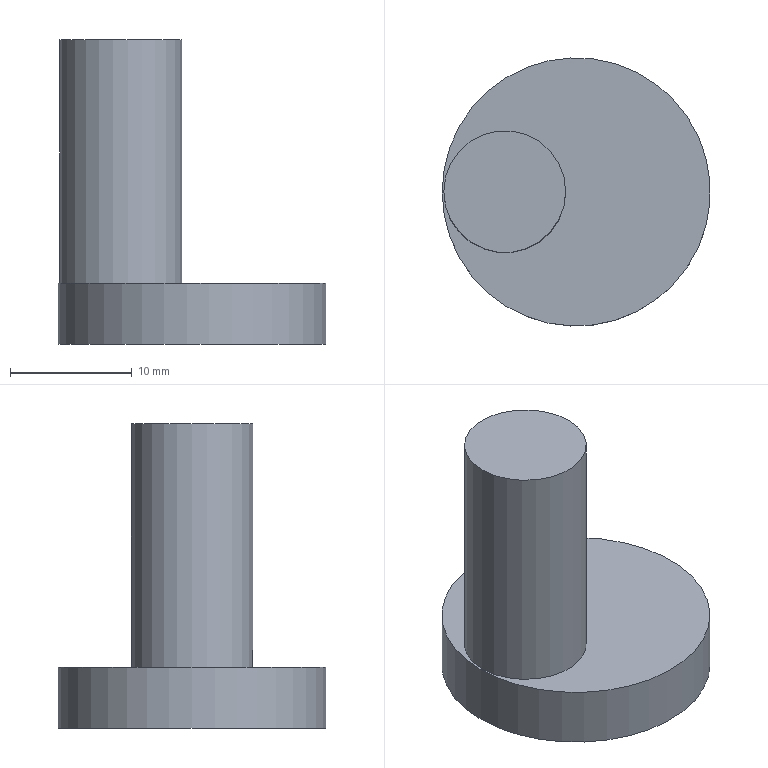Part | STEP file | CMT7E v7 | 1 solid | 5 faces | box 22 x 22 x 25 mm | volume 3472 mm3 | plane 3 | cylinder 2 | commonest cylinder face diameters 10 x1 22 x1
STEP:
#1=CARTESIAN_POINT('',(0.,0.,0.));
#2=DIRECTION('',(0.,0.,1.));
#3=DIRECTION('',(1.,0.,0.));
#4=AXIS2_PLACEMENT_3D('',#1,#2,#3);
#5=CARTESIAN_POINT('',(-79.635,-9.,16.));
#6=VERTEX_POINT('',#5);
#7=CARTESIAN_POINT('',(-68.635,-9.,16.));
#8=DIRECTION('',(0.,0.,1.));
#9=DIRECTION('',(-1.,0.,0.));
#10=AXIS2_PLACEMENT_3D('',#7,#8,#9);
#11=CIRCLE('',#10,11.);
#12=CARTESIAN_POINT('',(-68.635,-9.,16.));
#13=DIRECTION('',(0.,0.,1.));
#14=DIRECTION('',(-1.,0.,0.));
#15=AXIS2_PLACEMENT_3D('',#12,#13,#14);
#16=PLANE('',#15);
#17=CARTESIAN_POINT('',(0.,0.));
#18=DIRECTION('',(1.,0.));
#19=AXIS2_PLACEMENT_2D('',#17,#18);
#20=CIRCLE('',#19,11.);
#21=(GEOMETRIC_REPRESENTATION_CONTEXT(2)PARAMETRIC_REPRESENTATION_CONTEXT()REPRESENTATION_CONTEXT('',''));
#22=DEFINITIONAL_REPRESENTATION('',(#20),#21);
#23=PCURVE('',#16,#22);
#24=CARTESIAN_POINT('',(-68.635,-9.,16.));
#25=DIRECTION('',(0.,0.,1.));
#26=DIRECTION('',(-1.,0.,0.));
#27=AXIS2_PLACEMENT_3D('',#24,#25,#26);
#28=CYLINDRICAL_SURFACE('',#27,11.);
#29=CARTESIAN_POINT('',(0.,0.));
#30=DIRECTION('',(1.,0.));
#31=VECTOR('',#30,1.);
#32=LINE('',#29,#31);
#33=(GEOMETRIC_REPRESENTATION_CONTEXT(2)PARAMETRIC_REPRESENTATION_CONTEXT()REPRESENTATION_CONTEXT('',''));
#34=DEFINITIONAL_REPRESENTATION('',(#32),#33);
#35=PCURVE('',#28,#34);
#36=SURFACE_CURVE('',#11,(#23,#35),.PCURVE_S1.);
#37=EDGE_CURVE('',#6,#6,#36,.T.);
#38=ORIENTED_EDGE('',*,*,#37,.F.);
#39=EDGE_LOOP('',(#38));
#40=FACE_BOUND('',#39,.T.);
#41=ADVANCED_FACE('',(#40),#16,.F.);
#42=CARTESIAN_POINT('',(-79.5,-9.,21.));
#43=VERTEX_POINT('',#42);
#44=CARTESIAN_POINT('',(-74.5,-9.,21.));
#45=DIRECTION('',(0.,0.,-1.));
#46=DIRECTION('',(-1.,0.,0.));
#47=AXIS2_PLACEMENT_3D('',#44,#45,#46);
#48=CIRCLE('',#47,5.);
#49=CARTESIAN_POINT('',(-68.635,-9.,21.));
#50=DIRECTION('',(0.,0.,1.));
#51=DIRECTION('',(-1.,0.,0.));
#52=AXIS2_PLACEMENT_3D('',#49,#50,#51);
#53=PLANE('',#52);
#54=CARTESIAN_POINT('',(10.865,0.000000134));
#55=CARTESIAN_POINT('',(10.865,-8.66));
#56=CARTESIAN_POINT('',(3.365,-4.33));
#57=CARTESIAN_POINT('',(-4.135,0.000000134));
#58=CARTESIAN_POINT('',(3.365,4.33));
#59=CARTESIAN_POINT('',(10.865,8.66));
#60=CARTESIAN_POINT('',(10.865,0.000000134));
#61=(BOUNDED_CURVE()B_SPLINE_CURVE(2,(#54,#55,#56,#57,#58,#59,#60),.UNSPECIFIED.,.T.,.F.)B_SPLINE_CURVE_WITH_KNOTS((1,2,2,2,2,1),(-2.094,0.,2.094,4.189,6.283,8.378),.UNSPECIFIED.)CURVE()GEOMETRIC_REPRESENTATION_ITEM()RATIONAL_B_SPLINE_CURVE((1.,0.5,1.,0.5,1.,0.5,1.))REPRESENTATION_ITEM(''));
#62=(GEOMETRIC_REPRESENTATION_CONTEXT(2)PARAMETRIC_REPRESENTATION_CONTEXT()REPRESENTATION_CONTEXT('',''));
#63=DEFINITIONAL_REPRESENTATION('',(#61),#62);
#64=PCURVE('',#53,#63);
#65=CARTESIAN_POINT('',(-74.5,-9.,21.));
#66=DIRECTION('',(0.,0.,1.));
#67=DIRECTION('',(-1.,0.,0.));
#68=AXIS2_PLACEMENT_3D('',#65,#66,#67);
#69=CYLINDRICAL_SURFACE('',#68,5.);
#70=CARTESIAN_POINT('',(6.283,0.));
#71=DIRECTION('',(-1.,0.));
#72=VECTOR('',#71,1.);
#73=LINE('',#70,#72);
#74=(GEOMETRIC_REPRESENTATION_CONTEXT(2)PARAMETRIC_REPRESENTATION_CONTEXT()REPRESENTATION_CONTEXT('',''));
#75=DEFINITIONAL_REPRESENTATION('',(#73),#74);
#76=PCURVE('',#69,#75);
#77=SURFACE_CURVE('',#48,(#64,#76),.PCURVE_S1.);
#78=EDGE_CURVE('',#43,#43,#77,.T.);
#79=ORIENTED_EDGE('',*,*,#78,.T.);
#80=EDGE_LOOP('',(#79));
#81=FACE_BOUND('',#80,.T.);
#82=CARTESIAN_POINT('',(-79.635,-9.,21.));
#83=VERTEX_POINT('',#82);
#84=CARTESIAN_POINT('',(-68.635,-9.,21.));
#85=DIRECTION('',(0.,0.,1.));
#86=DIRECTION('',(-1.,0.,0.));
#87=AXIS2_PLACEMENT_3D('',#84,#85,#86);
#88=CIRCLE('',#87,11.);
#89=CARTESIAN_POINT('',(0.,0.));
#90=DIRECTION('',(1.,0.));
#91=AXIS2_PLACEMENT_2D('',#89,#90);
#92=CIRCLE('',#91,11.);
#93=(GEOMETRIC_REPRESENTATION_CONTEXT(2)PARAMETRIC_REPRESENTATION_CONTEXT()REPRESENTATION_CONTEXT('',''));
#94=DEFINITIONAL_REPRESENTATION('',(#92),#93);
#95=PCURVE('',#53,#94);
#96=CARTESIAN_POINT('',(0.,5.));
#97=DIRECTION('',(1.,0.));
#98=VECTOR('',#97,1.);
#99=LINE('',#96,#98);
#100=(GEOMETRIC_REPRESENTATION_CONTEXT(2)PARAMETRIC_REPRESENTATION_CONTEXT()REPRESENTATION_CONTEXT('',''));
#101=DEFINITIONAL_REPRESENTATION('',(#99),#100);
#102=PCURVE('',#28,#101);
#103=SURFACE_CURVE('',#88,(#95,#102),.PCURVE_S1.);
#104=EDGE_CURVE('',#83,#83,#103,.T.);
#105=ORIENTED_EDGE('',*,*,#104,.T.);
#106=EDGE_LOOP('',(#105));
#107=FACE_BOUND('',#106,.T.);
#108=ADVANCED_FACE('',(#81,#107),#53,.T.);
#109=ORIENTED_EDGE('',*,*,#37,.T.);
#110=CARTESIAN_POINT('',(-79.635,-9.,16.));
#111=CARTESIAN_POINT('',(-79.635,-9.,21.));
#112=B_SPLINE_CURVE_WITH_KNOTS('',1,(#110,#111),.UNSPECIFIED.,.F.,.F.,(2,2),(0.,5.),.PIECEWISE_BEZIER_KNOTS.);
#113=CARTESIAN_POINT('',(6.283,0.));
#114=DIRECTION('',(0.,1.));
#115=VECTOR('',#114,1.);
#116=LINE('',#113,#115);
#117=(GEOMETRIC_REPRESENTATION_CONTEXT(2)PARAMETRIC_REPRESENTATION_CONTEXT()REPRESENTATION_CONTEXT('',''));
#118=DEFINITIONAL_REPRESENTATION('',(#116),#117);
#119=PCURVE('',#28,#118);
#120=CARTESIAN_POINT('',(0.,0.));
#121=DIRECTION('',(0.,1.));
#122=VECTOR('',#121,1.);
#123=LINE('',#120,#122);
#124=(GEOMETRIC_REPRESENTATION_CONTEXT(2)PARAMETRIC_REPRESENTATION_CONTEXT()REPRESENTATION_CONTEXT('',''));
#125=DEFINITIONAL_REPRESENTATION('',(#123),#124);
#126=PCURVE('',#28,#125);
#127=SEAM_CURVE('',#112,(#119,#126),.PCURVE_S1.);
#128=EDGE_CURVE('',#6,#83,#127,.T.);
#129=ORIENTED_EDGE('',*,*,#128,.T.);
#130=ORIENTED_EDGE('',*,*,#104,.F.);
#131=ORIENTED_EDGE('',*,*,#128,.F.);
#132=EDGE_LOOP('',(#109,#129,#130,#131));
#133=FACE_BOUND('',#132,.T.);
#134=ADVANCED_FACE('',(#133),#28,.T.);
#135=CARTESIAN_POINT('',(-79.5,-9.,41.));
#136=VERTEX_POINT('',#135);
#137=CARTESIAN_POINT('',(-74.5,-9.,41.));
#138=DIRECTION('',(0.,0.,1.));
#139=DIRECTION('',(-1.,0.,0.));
#140=AXIS2_PLACEMENT_3D('',#137,#138,#139);
#141=CIRCLE('',#140,5.);
#142=CARTESIAN_POINT('',(-74.5,-9.,41.));
#143=DIRECTION('',(0.,0.,1.));
#144=DIRECTION('',(-1.,0.,0.));
#145=AXIS2_PLACEMENT_3D('',#142,#143,#144);
#146=PLANE('',#145);
#147=CARTESIAN_POINT('',(0.,0.));
#148=DIRECTION('',(1.,0.));
#149=AXIS2_PLACEMENT_2D('',#147,#148);
#150=CIRCLE('',#149,5.);
#151=(GEOMETRIC_REPRESENTATION_CONTEXT(2)PARAMETRIC_REPRESENTATION_CONTEXT()REPRESENTATION_CONTEXT('',''));
#152=DEFINITIONAL_REPRESENTATION('',(#150),#151);
#153=PCURVE('',#146,#152);
#154=CARTESIAN_POINT('',(0.,20.));
#155=DIRECTION('',(1.,0.));
#156=VECTOR('',#155,1.);
#157=LINE('',#154,#156);
#158=(GEOMETRIC_REPRESENTATION_CONTEXT(2)PARAMETRIC_REPRESENTATION_CONTEXT()REPRESENTATION_CONTEXT('',''));
#159=DEFINITIONAL_REPRESENTATION('',(#157),#158);
#160=PCURVE('',#69,#159);
#161=SURFACE_CURVE('',#141,(#153,#160),.PCURVE_S1.);
#162=EDGE_CURVE('',#136,#136,#161,.T.);
#163=ORIENTED_EDGE('',*,*,#162,.T.);
#164=EDGE_LOOP('',(#163));
#165=FACE_BOUND('',#164,.T.);
#166=ADVANCED_FACE('',(#165),#146,.T.);
#167=ORIENTED_EDGE('',*,*,#78,.F.);
#168=CARTESIAN_POINT('',(-79.5,-9.,21.));
#169=CARTESIAN_POINT('',(-79.5,-9.,41.));
#170=B_SPLINE_CURVE_WITH_KNOTS('',1,(#168,#169),.UNSPECIFIED.,.F.,.F.,(2,2),(0.,20.),.PIECEWISE_BEZIER_KNOTS.);
#171=CARTESIAN_POINT('',(6.283,0.));
#172=DIRECTION('',(0.,1.));
#173=VECTOR('',#172,1.);
#174=LINE('',#171,#173);
#175=(GEOMETRIC_REPRESENTATION_CONTEXT(2)PARAMETRIC_REPRESENTATION_CONTEXT()REPRESENTATION_CONTEXT('',''));
#176=DEFINITIONAL_REPRESENTATION('',(#174),#175);
#177=PCURVE('',#69,#176);
#178=CARTESIAN_POINT('',(0.,0.));
#179=DIRECTION('',(0.,1.));
#180=VECTOR('',#179,1.);
#181=LINE('',#178,#180);
#182=(GEOMETRIC_REPRESENTATION_CONTEXT(2)PARAMETRIC_REPRESENTATION_CONTEXT()REPRESENTATION_CONTEXT('',''));
#183=DEFINITIONAL_REPRESENTATION('',(#181),#182);
#184=PCURVE('',#69,#183);
#185=SEAM_CURVE('',#170,(#177,#184),.PCURVE_S1.);
#186=EDGE_CURVE('',#43,#136,#185,.T.);
#187=ORIENTED_EDGE('',*,*,#186,.T.);
#188=ORIENTED_EDGE('',*,*,#162,.F.);
#189=ORIENTED_EDGE('',*,*,#186,.F.);
#190=EDGE_LOOP('',(#167,#187,#188,#189));
#191=FACE_BOUND('',#190,.T.);
#192=ADVANCED_FACE('',(#191),#69,.T.);
#193=CLOSED_SHELL('',(#41,#108,#134,#166,#192));
#194=MANIFOLD_SOLID_BREP('',#193);
#195=(LENGTH_UNIT()NAMED_UNIT(*)SI_UNIT(.MILLI.,.METRE.));
#196=UNCERTAINTY_MEASURE_WITH_UNIT(LENGTH_MEASURE(0.0000001),#195,'','');
#197=(NAMED_UNIT(*)PLANE_ANGLE_UNIT()SI_UNIT($,.RADIAN.));
#198=(NAMED_UNIT(*)SI_UNIT($,.STERADIAN.)SOLID_ANGLE_UNIT());
#199=(GEOMETRIC_REPRESENTATION_CONTEXT(3)GLOBAL_UNCERTAINTY_ASSIGNED_CONTEXT((#196))GLOBAL_UNIT_ASSIGNED_CONTEXT((#195,#197,#198))REPRESENTATION_CONTEXT('',''));
#200=ADVANCED_BREP_SHAPE_REPRESENTATION('',(#4,#194),#199);